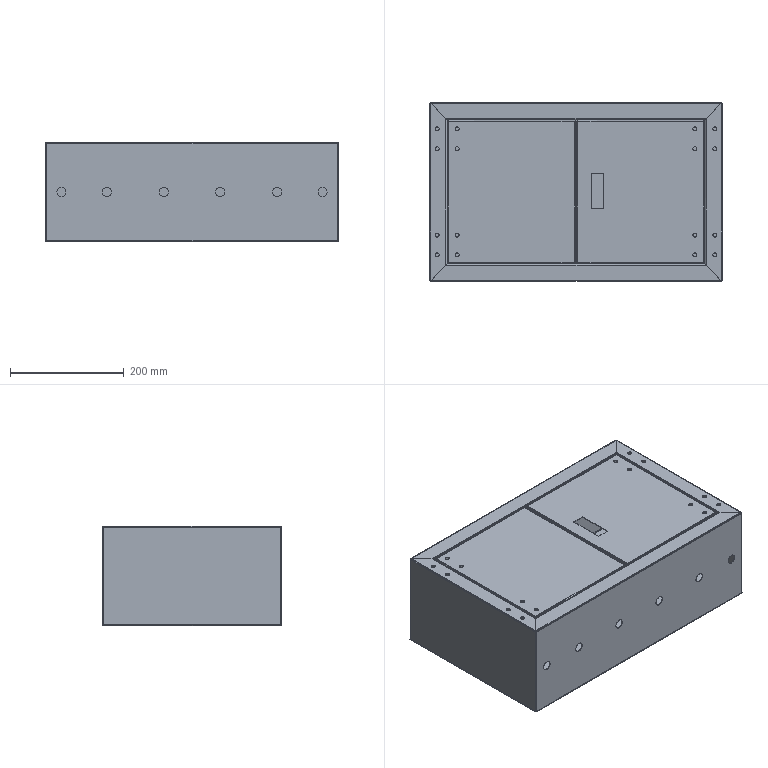Part | 7 solids | 412 faces | box 515 x 315 x 175 mm | volume 828776 mm3 | plane 194 | cylinder 152 | spline 62 | torus 4 | commonest cylinder face diameters 1.473 x32 3.873 x32 7 x32 10 x12 16 x12 2 x8